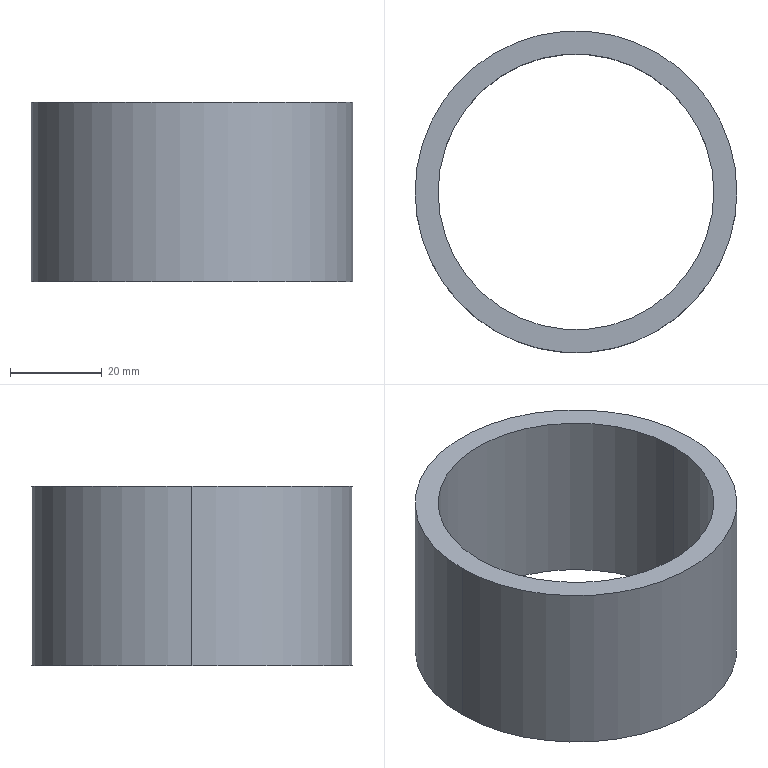Part | STEP file | 05-Spacer 1 | 1 solid | 6 faces | box 70 x 70 x 39 mm | volume 39820 mm3 | cylinder 4 | plane 2 | commonest cylinder face diameters 60 x2 70 x2
STEP:
#1=CARTESIAN_POINT('',(0.,0.,0.));
#2=DIRECTION('',(0.,0.,1.));
#3=DIRECTION('',(1.,0.,0.));
#4=AXIS2_PLACEMENT_3D('',#1,#2,#3);
#5=CARTESIAN_POINT('',(-30.,0.,39.));
#6=VERTEX_POINT('',#5);
#7=CARTESIAN_POINT('',(-30.,0.,0.));
#8=VERTEX_POINT('',#7);
#9=CARTESIAN_POINT('',(-30.,0.,39.));
#10=DIRECTION('',(0.,0.,-1.));
#11=VECTOR('',#10,1.);
#12=LINE('',#9,#11);
#13=CARTESIAN_POINT('',(0.,0.,39.));
#14=DIRECTION('',(0.,0.,-1.));
#15=DIRECTION('',(-1.,0.,0.));
#16=AXIS2_PLACEMENT_3D('',#13,#14,#15);
#17=CYLINDRICAL_SURFACE('',#16,30.);
#18=CARTESIAN_POINT('',(6.283,0.));
#19=DIRECTION('',(0.,1.));
#20=VECTOR('',#19,1.);
#21=LINE('',#18,#20);
#22=(GEOMETRIC_REPRESENTATION_CONTEXT(2)PARAMETRIC_REPRESENTATION_CONTEXT()REPRESENTATION_CONTEXT('',''));
#23=DEFINITIONAL_REPRESENTATION('',(#21),#22);
#24=PCURVE('',#17,#23);
#25=CARTESIAN_POINT('',(0.,0.,39.));
#26=DIRECTION('',(0.,0.,-1.));
#27=DIRECTION('',(-1.,0.,0.));
#28=AXIS2_PLACEMENT_3D('',#25,#26,#27);
#29=CYLINDRICAL_SURFACE('',#28,30.);
#30=CARTESIAN_POINT('',(0.,0.));
#31=DIRECTION('',(0.,1.));
#32=VECTOR('',#31,1.);
#33=LINE('',#30,#32);
#34=(GEOMETRIC_REPRESENTATION_CONTEXT(2)PARAMETRIC_REPRESENTATION_CONTEXT()REPRESENTATION_CONTEXT('',''));
#35=DEFINITIONAL_REPRESENTATION('',(#33),#34);
#36=PCURVE('',#29,#35);
#37=SURFACE_CURVE('',#12,(#24,#36),.PCURVE_S1.);
#38=EDGE_CURVE('',#6,#8,#37,.T.);
#39=ORIENTED_EDGE('',*,*,#38,.T.);
#40=CARTESIAN_POINT('',(30.,0.,0.));
#41=VERTEX_POINT('',#40);
#42=CARTESIAN_POINT('',(0.,0.,0.));
#43=DIRECTION('',(0.,0.,1.));
#44=DIRECTION('',(1.,0.,0.));
#45=AXIS2_PLACEMENT_3D('',#42,#43,#44);
#46=CIRCLE('',#45,30.);
#47=CARTESIAN_POINT('',(9.425,39.));
#48=DIRECTION('',(-1.,0.));
#49=VECTOR('',#48,1.);
#50=LINE('',#47,#49);
#51=(GEOMETRIC_REPRESENTATION_CONTEXT(2)PARAMETRIC_REPRESENTATION_CONTEXT()REPRESENTATION_CONTEXT('',''));
#52=DEFINITIONAL_REPRESENTATION('',(#50),#51);
#53=PCURVE('',#17,#52);
#54=CARTESIAN_POINT('',(0.,0.,0.));
#55=DIRECTION('',(0.,0.,1.));
#56=DIRECTION('',(1.,0.,0.));
#57=AXIS2_PLACEMENT_3D('',#54,#55,#56);
#58=PLANE('',#57);
#59=CARTESIAN_POINT('',(0.,0.));
#60=DIRECTION('',(1.,0.));
#61=AXIS2_PLACEMENT_2D('',#59,#60);
#62=CIRCLE('',#61,30.);
#63=(GEOMETRIC_REPRESENTATION_CONTEXT(2)PARAMETRIC_REPRESENTATION_CONTEXT()REPRESENTATION_CONTEXT('',''));
#64=DEFINITIONAL_REPRESENTATION('',(#62),#63);
#65=PCURVE('',#58,#64);
#66=SURFACE_CURVE('',#46,(#53,#65),.PCURVE_S1.);
#67=EDGE_CURVE('',#8,#41,#66,.T.);
#68=ORIENTED_EDGE('',*,*,#67,.T.);
#69=CARTESIAN_POINT('',(30.,0.,39.));
#70=VERTEX_POINT('',#69);
#71=CARTESIAN_POINT('',(30.,0.,39.));
#72=DIRECTION('',(0.,0.,-1.));
#73=VECTOR('',#72,1.);
#74=LINE('',#71,#73);
#75=CARTESIAN_POINT('',(3.142,0.));
#76=DIRECTION('',(0.,1.));
#77=VECTOR('',#76,1.);
#78=LINE('',#75,#77);
#79=(GEOMETRIC_REPRESENTATION_CONTEXT(2)PARAMETRIC_REPRESENTATION_CONTEXT()REPRESENTATION_CONTEXT('',''));
#80=DEFINITIONAL_REPRESENTATION('',(#78),#79);
#81=PCURVE('',#17,#80);
#82=CARTESIAN_POINT('',(3.142,0.));
#83=DIRECTION('',(0.,1.));
#84=VECTOR('',#83,1.);
#85=LINE('',#82,#84);
#86=(GEOMETRIC_REPRESENTATION_CONTEXT(2)PARAMETRIC_REPRESENTATION_CONTEXT()REPRESENTATION_CONTEXT('',''));
#87=DEFINITIONAL_REPRESENTATION('',(#85),#86);
#88=PCURVE('',#29,#87);
#89=SURFACE_CURVE('',#74,(#81,#88),.PCURVE_S1.);
#90=EDGE_CURVE('',#70,#41,#89,.T.);
#91=ORIENTED_EDGE('',*,*,#90,.F.);
#92=CARTESIAN_POINT('',(0.,0.,39.));
#93=DIRECTION('',(0.,0.,1.));
#94=DIRECTION('',(1.,0.,0.));
#95=AXIS2_PLACEMENT_3D('',#92,#93,#94);
#96=CIRCLE('',#95,30.);
#97=CARTESIAN_POINT('',(9.425,0.));
#98=DIRECTION('',(-1.,0.));
#99=VECTOR('',#98,1.);
#100=LINE('',#97,#99);
#101=(GEOMETRIC_REPRESENTATION_CONTEXT(2)PARAMETRIC_REPRESENTATION_CONTEXT()REPRESENTATION_CONTEXT('',''));
#102=DEFINITIONAL_REPRESENTATION('',(#100),#101);
#103=PCURVE('',#17,#102);
#104=CARTESIAN_POINT('',(0.,0.,39.));
#105=DIRECTION('',(0.,0.,1.));
#106=DIRECTION('',(1.,0.,0.));
#107=AXIS2_PLACEMENT_3D('',#104,#105,#106);
#108=PLANE('',#107);
#109=CARTESIAN_POINT('',(0.,0.));
#110=DIRECTION('',(1.,0.));
#111=AXIS2_PLACEMENT_2D('',#109,#110);
#112=CIRCLE('',#111,30.);
#113=(GEOMETRIC_REPRESENTATION_CONTEXT(2)PARAMETRIC_REPRESENTATION_CONTEXT()REPRESENTATION_CONTEXT('',''));
#114=DEFINITIONAL_REPRESENTATION('',(#112),#113);
#115=PCURVE('',#108,#114);
#116=SURFACE_CURVE('',#96,(#103,#115),.PCURVE_S1.);
#117=EDGE_CURVE('',#6,#70,#116,.T.);
#118=ORIENTED_EDGE('',*,*,#117,.F.);
#119=EDGE_LOOP('',(#39,#68,#91,#118));
#120=FACE_BOUND('',#119,.F.);
#121=ADVANCED_FACE('',(#120),#17,.F.);
#122=CARTESIAN_POINT('',(35.,0.,39.));
#123=VERTEX_POINT('',#122);
#124=CARTESIAN_POINT('',(-35.,0.,39.));
#125=VERTEX_POINT('',#124);
#126=CARTESIAN_POINT('',(0.,0.,39.));
#127=DIRECTION('',(0.,0.,1.));
#128=DIRECTION('',(1.,0.,0.));
#129=AXIS2_PLACEMENT_3D('',#126,#127,#128);
#130=CIRCLE('',#129,35.);
#131=CARTESIAN_POINT('',(0.,0.,39.));
#132=DIRECTION('',(0.,0.,-1.));
#133=DIRECTION('',(-1.,0.,0.));
#134=AXIS2_PLACEMENT_3D('',#131,#132,#133);
#135=CYLINDRICAL_SURFACE('',#134,35.);
#136=CARTESIAN_POINT('',(3.142,0.));
#137=DIRECTION('',(-1.,0.));
#138=VECTOR('',#137,1.);
#139=LINE('',#136,#138);
#140=(GEOMETRIC_REPRESENTATION_CONTEXT(2)PARAMETRIC_REPRESENTATION_CONTEXT()REPRESENTATION_CONTEXT('',''));
#141=DEFINITIONAL_REPRESENTATION('',(#139),#140);
#142=PCURVE('',#135,#141);
#143=CARTESIAN_POINT('',(0.,0.));
#144=DIRECTION('',(1.,0.));
#145=AXIS2_PLACEMENT_2D('',#143,#144);
#146=CIRCLE('',#145,35.);
#147=(GEOMETRIC_REPRESENTATION_CONTEXT(2)PARAMETRIC_REPRESENTATION_CONTEXT()REPRESENTATION_CONTEXT('',''));
#148=DEFINITIONAL_REPRESENTATION('',(#146),#147);
#149=PCURVE('',#108,#148);
#150=SURFACE_CURVE('',#130,(#142,#149),.PCURVE_S1.);
#151=EDGE_CURVE('',#123,#125,#150,.T.);
#152=ORIENTED_EDGE('',*,*,#151,.F.);
#153=CARTESIAN_POINT('',(35.,0.,0.));
#154=VERTEX_POINT('',#153);
#155=CARTESIAN_POINT('',(35.,0.,39.));
#156=DIRECTION('',(0.,0.,-1.));
#157=VECTOR('',#156,1.);
#158=LINE('',#155,#157);
#159=CARTESIAN_POINT('',(3.142,0.));
#160=DIRECTION('',(0.,1.));
#161=VECTOR('',#160,1.);
#162=LINE('',#159,#161);
#163=(GEOMETRIC_REPRESENTATION_CONTEXT(2)PARAMETRIC_REPRESENTATION_CONTEXT()REPRESENTATION_CONTEXT('',''));
#164=DEFINITIONAL_REPRESENTATION('',(#162),#163);
#165=PCURVE('',#135,#164);
#166=CARTESIAN_POINT('',(0.,0.,39.));
#167=DIRECTION('',(0.,0.,-1.));
#168=DIRECTION('',(-1.,0.,0.));
#169=AXIS2_PLACEMENT_3D('',#166,#167,#168);
#170=CYLINDRICAL_SURFACE('',#169,35.);
#171=CARTESIAN_POINT('',(3.142,0.));
#172=DIRECTION('',(0.,1.));
#173=VECTOR('',#172,1.);
#174=LINE('',#171,#173);
#175=(GEOMETRIC_REPRESENTATION_CONTEXT(2)PARAMETRIC_REPRESENTATION_CONTEXT()REPRESENTATION_CONTEXT('',''));
#176=DEFINITIONAL_REPRESENTATION('',(#174),#175);
#177=PCURVE('',#170,#176);
#178=SURFACE_CURVE('',#158,(#165,#177),.PCURVE_S1.);
#179=EDGE_CURVE('',#123,#154,#178,.T.);
#180=ORIENTED_EDGE('',*,*,#179,.T.);
#181=CARTESIAN_POINT('',(-35.,0.,0.));
#182=VERTEX_POINT('',#181);
#183=CARTESIAN_POINT('',(0.,0.,0.));
#184=DIRECTION('',(0.,0.,1.));
#185=DIRECTION('',(1.,0.,0.));
#186=AXIS2_PLACEMENT_3D('',#183,#184,#185);
#187=CIRCLE('',#186,35.);
#188=CARTESIAN_POINT('',(3.142,39.));
#189=DIRECTION('',(-1.,0.));
#190=VECTOR('',#189,1.);
#191=LINE('',#188,#190);
#192=(GEOMETRIC_REPRESENTATION_CONTEXT(2)PARAMETRIC_REPRESENTATION_CONTEXT()REPRESENTATION_CONTEXT('',''));
#193=DEFINITIONAL_REPRESENTATION('',(#191),#192);
#194=PCURVE('',#135,#193);
#195=CARTESIAN_POINT('',(0.,0.));
#196=DIRECTION('',(1.,0.));
#197=AXIS2_PLACEMENT_2D('',#195,#196);
#198=CIRCLE('',#197,35.);
#199=(GEOMETRIC_REPRESENTATION_CONTEXT(2)PARAMETRIC_REPRESENTATION_CONTEXT()REPRESENTATION_CONTEXT('',''));
#200=DEFINITIONAL_REPRESENTATION('',(#198),#199);
#201=PCURVE('',#58,#200);
#202=SURFACE_CURVE('',#187,(#194,#201),.PCURVE_S1.);
#203=EDGE_CURVE('',#154,#182,#202,.T.);
#204=ORIENTED_EDGE('',*,*,#203,.T.);
#205=CARTESIAN_POINT('',(-35.,0.,39.));
#206=DIRECTION('',(0.,0.,-1.));
#207=VECTOR('',#206,1.);
#208=LINE('',#205,#207);
#209=CARTESIAN_POINT('',(0.,0.));
#210=DIRECTION('',(0.,1.));
#211=VECTOR('',#210,1.);
#212=LINE('',#209,#211);
#213=(GEOMETRIC_REPRESENTATION_CONTEXT(2)PARAMETRIC_REPRESENTATION_CONTEXT()REPRESENTATION_CONTEXT('',''));
#214=DEFINITIONAL_REPRESENTATION('',(#212),#213);
#215=PCURVE('',#135,#214);
#216=CARTESIAN_POINT('',(6.283,0.));
#217=DIRECTION('',(0.,1.));
#218=VECTOR('',#217,1.);
#219=LINE('',#216,#218);
#220=(GEOMETRIC_REPRESENTATION_CONTEXT(2)PARAMETRIC_REPRESENTATION_CONTEXT()REPRESENTATION_CONTEXT('',''));
#221=DEFINITIONAL_REPRESENTATION('',(#219),#220);
#222=PCURVE('',#170,#221);
#223=SURFACE_CURVE('',#208,(#215,#222),.PCURVE_S1.);
#224=EDGE_CURVE('',#125,#182,#223,.T.);
#225=ORIENTED_EDGE('',*,*,#224,.F.);
#226=EDGE_LOOP('',(#152,#180,#204,#225));
#227=FACE_BOUND('',#226,.T.);
#228=ADVANCED_FACE('',(#227),#135,.T.);
#229=CARTESIAN_POINT('',(0.,0.,39.));
#230=DIRECTION('',(0.,0.,1.));
#231=DIRECTION('',(1.,0.,0.));
#232=AXIS2_PLACEMENT_3D('',#229,#230,#231);
#233=CIRCLE('',#232,35.);
#234=CARTESIAN_POINT('',(0.,0.));
#235=DIRECTION('',(1.,0.));
#236=AXIS2_PLACEMENT_2D('',#234,#235);
#237=CIRCLE('',#236,35.);
#238=(GEOMETRIC_REPRESENTATION_CONTEXT(2)PARAMETRIC_REPRESENTATION_CONTEXT()REPRESENTATION_CONTEXT('',''));
#239=DEFINITIONAL_REPRESENTATION('',(#237),#238);
#240=PCURVE('',#108,#239);
#241=CARTESIAN_POINT('',(9.425,0.));
#242=DIRECTION('',(-1.,0.));
#243=VECTOR('',#242,1.);
#244=LINE('',#241,#243);
#245=(GEOMETRIC_REPRESENTATION_CONTEXT(2)PARAMETRIC_REPRESENTATION_CONTEXT()REPRESENTATION_CONTEXT('',''));
#246=DEFINITIONAL_REPRESENTATION('',(#244),#245);
#247=PCURVE('',#170,#246);
#248=SURFACE_CURVE('',#233,(#240,#247),.PCURVE_S1.);
#249=EDGE_CURVE('',#125,#123,#248,.T.);
#250=ORIENTED_EDGE('',*,*,#249,.T.);
#251=ORIENTED_EDGE('',*,*,#151,.T.);
#252=EDGE_LOOP('',(#250,#251));
#253=FACE_BOUND('',#252,.T.);
#254=ORIENTED_EDGE('',*,*,#117,.F.);
#255=CARTESIAN_POINT('',(0.,0.,39.));
#256=DIRECTION('',(0.,0.,1.));
#257=DIRECTION('',(1.,0.,0.));
#258=AXIS2_PLACEMENT_3D('',#255,#256,#257);
#259=CIRCLE('',#258,30.);
#260=CARTESIAN_POINT('',(0.,0.));
#261=DIRECTION('',(1.,0.));
#262=AXIS2_PLACEMENT_2D('',#260,#261);
#263=CIRCLE('',#262,30.);
#264=(GEOMETRIC_REPRESENTATION_CONTEXT(2)PARAMETRIC_REPRESENTATION_CONTEXT()REPRESENTATION_CONTEXT('',''));
#265=DEFINITIONAL_REPRESENTATION('',(#263),#264);
#266=PCURVE('',#108,#265);
#267=CARTESIAN_POINT('',(3.142,0.));
#268=DIRECTION('',(-1.,0.));
#269=VECTOR('',#268,1.);
#270=LINE('',#267,#269);
#271=(GEOMETRIC_REPRESENTATION_CONTEXT(2)PARAMETRIC_REPRESENTATION_CONTEXT()REPRESENTATION_CONTEXT('',''));
#272=DEFINITIONAL_REPRESENTATION('',(#270),#271);
#273=PCURVE('',#29,#272);
#274=SURFACE_CURVE('',#259,(#266,#273),.PCURVE_S1.);
#275=EDGE_CURVE('',#70,#6,#274,.T.);
#276=ORIENTED_EDGE('',*,*,#275,.F.);
#277=EDGE_LOOP('',(#254,#276));
#278=FACE_BOUND('',#277,.T.);
#279=ADVANCED_FACE('',(#253,#278),#108,.T.);
#280=CARTESIAN_POINT('',(0.,0.,0.));
#281=DIRECTION('',(0.,0.,1.));
#282=DIRECTION('',(1.,0.,0.));
#283=AXIS2_PLACEMENT_3D('',#280,#281,#282);
#284=CIRCLE('',#283,35.);
#285=CARTESIAN_POINT('',(0.,0.));
#286=DIRECTION('',(1.,0.));
#287=AXIS2_PLACEMENT_2D('',#285,#286);
#288=CIRCLE('',#287,35.);
#289=(GEOMETRIC_REPRESENTATION_CONTEXT(2)PARAMETRIC_REPRESENTATION_CONTEXT()REPRESENTATION_CONTEXT('',''));
#290=DEFINITIONAL_REPRESENTATION('',(#288),#289);
#291=PCURVE('',#58,#290);
#292=CARTESIAN_POINT('',(9.425,39.));
#293=DIRECTION('',(-1.,0.));
#294=VECTOR('',#293,1.);
#295=LINE('',#292,#294);
#296=(GEOMETRIC_REPRESENTATION_CONTEXT(2)PARAMETRIC_REPRESENTATION_CONTEXT()REPRESENTATION_CONTEXT('',''));
#297=DEFINITIONAL_REPRESENTATION('',(#295),#296);
#298=PCURVE('',#170,#297);
#299=SURFACE_CURVE('',#284,(#291,#298),.PCURVE_S1.);
#300=EDGE_CURVE('',#182,#154,#299,.T.);
#301=ORIENTED_EDGE('',*,*,#300,.F.);
#302=ORIENTED_EDGE('',*,*,#203,.F.);
#303=EDGE_LOOP('',(#301,#302));
#304=FACE_BOUND('',#303,.T.);
#305=ORIENTED_EDGE('',*,*,#67,.T.);
#306=CARTESIAN_POINT('',(0.,0.,0.));
#307=DIRECTION('',(0.,0.,1.));
#308=DIRECTION('',(1.,0.,0.));
#309=AXIS2_PLACEMENT_3D('',#306,#307,#308);
#310=CIRCLE('',#309,30.);
#311=CARTESIAN_POINT('',(0.,0.));
#312=DIRECTION('',(1.,0.));
#313=AXIS2_PLACEMENT_2D('',#311,#312);
#314=CIRCLE('',#313,30.);
#315=(GEOMETRIC_REPRESENTATION_CONTEXT(2)PARAMETRIC_REPRESENTATION_CONTEXT()REPRESENTATION_CONTEXT('',''));
#316=DEFINITIONAL_REPRESENTATION('',(#314),#315);
#317=PCURVE('',#58,#316);
#318=CARTESIAN_POINT('',(3.142,39.));
#319=DIRECTION('',(-1.,0.));
#320=VECTOR('',#319,1.);
#321=LINE('',#318,#320);
#322=(GEOMETRIC_REPRESENTATION_CONTEXT(2)PARAMETRIC_REPRESENTATION_CONTEXT()REPRESENTATION_CONTEXT('',''));
#323=DEFINITIONAL_REPRESENTATION('',(#321),#322);
#324=PCURVE('',#29,#323);
#325=SURFACE_CURVE('',#310,(#317,#324),.PCURVE_S1.);
#326=EDGE_CURVE('',#41,#8,#325,.T.);
#327=ORIENTED_EDGE('',*,*,#326,.T.);
#328=EDGE_LOOP('',(#305,#327));
#329=FACE_BOUND('',#328,.T.);
#330=ADVANCED_FACE('',(#304,#329),#58,.F.);
#331=ORIENTED_EDGE('',*,*,#179,.F.);
#332=ORIENTED_EDGE('',*,*,#249,.F.);
#333=ORIENTED_EDGE('',*,*,#224,.T.);
#334=ORIENTED_EDGE('',*,*,#300,.T.);
#335=EDGE_LOOP('',(#331,#332,#333,#334));
#336=FACE_BOUND('',#335,.T.);
#337=ADVANCED_FACE('',(#336),#170,.T.);
#338=ORIENTED_EDGE('',*,*,#326,.T.);
#339=ORIENTED_EDGE('',*,*,#38,.F.);
#340=ORIENTED_EDGE('',*,*,#275,.F.);
#341=ORIENTED_EDGE('',*,*,#90,.T.);
#342=EDGE_LOOP('',(#338,#339,#340,#341));
#343=FACE_BOUND('',#342,.F.);
#344=ADVANCED_FACE('',(#343),#29,.F.);
#345=CLOSED_SHELL('',(#121,#228,#279,#330,#337,#344));
#346=MANIFOLD_SOLID_BREP('',#345);
#347=(LENGTH_UNIT()NAMED_UNIT(*)SI_UNIT(.MILLI.,.METRE.));
#348=UNCERTAINTY_MEASURE_WITH_UNIT(LENGTH_MEASURE(0.0000001),#347,'','');
#349=(NAMED_UNIT(*)PLANE_ANGLE_UNIT()SI_UNIT($,.RADIAN.));
#350=(NAMED_UNIT(*)SI_UNIT($,.STERADIAN.)SOLID_ANGLE_UNIT());
#351=(GEOMETRIC_REPRESENTATION_CONTEXT(3)GLOBAL_UNCERTAINTY_ASSIGNED_CONTEXT((#348))GLOBAL_UNIT_ASSIGNED_CONTEXT((#347,#349,#350))REPRESENTATION_CONTEXT('',''));
#352=ADVANCED_BREP_SHAPE_REPRESENTATION('',(#4,#346),#351);